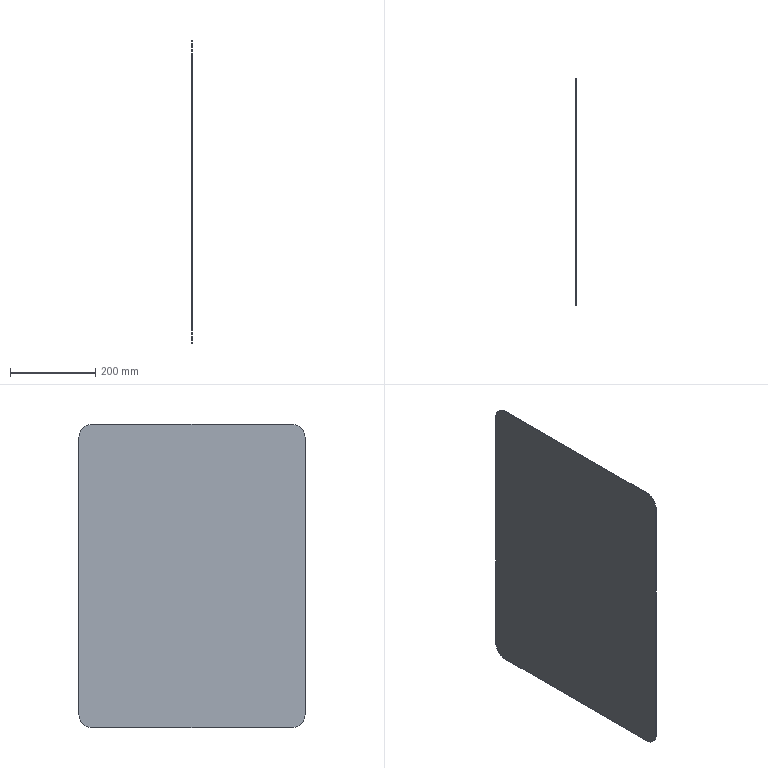Part | STEP file | 冲床-300配套压波_id1018_x_t | 1 solid | 10 faces | box 1.2 x 530 x 710 mm | volume 450633 mm3 | plane 6 | cylinder 4 | commonest cylinder face diameters 60 x4
STEP:
#1=CARTESIAN_POINT('',(1160.,-265.,-725.));
#2=VERTEX_POINT('',#1);
#3=CARTESIAN_POINT('',(1160.,-265.,-75.));
#4=VERTEX_POINT('',#3);
#5=CARTESIAN_POINT('',(1160.,-265.,-755.));
#6=DIRECTION('',(0.,0.,1.));
#7=VECTOR('',#6,1.);
#8=LINE('',#5,#7);
#9=EDGE_CURVE('',#2,#4,#8,.T.);
#10=ORIENTED_EDGE('',*,*,#9,.T.);
#11=CARTESIAN_POINT('',(1158.8,-265.,-75.));
#12=VERTEX_POINT('',#11);
#13=CARTESIAN_POINT('',(1160.,-265.,-75.));
#14=DIRECTION('',(-1.,0.,0.));
#15=VECTOR('',#14,1.);
#16=LINE('',#13,#15);
#17=EDGE_CURVE('',#4,#12,#16,.T.);
#18=ORIENTED_EDGE('',*,*,#17,.T.);
#19=CARTESIAN_POINT('',(1158.8,-265.,-725.));
#20=VERTEX_POINT('',#19);
#21=CARTESIAN_POINT('',(1158.8,-265.,-755.));
#22=DIRECTION('',(0.,0.,1.));
#23=VECTOR('',#22,1.);
#24=LINE('',#21,#23);
#25=EDGE_CURVE('',#20,#12,#24,.T.);
#26=ORIENTED_EDGE('',*,*,#25,.F.);
#27=CARTESIAN_POINT('',(1160.,-265.,-725.));
#28=DIRECTION('',(1.,0.,0.));
#29=VECTOR('',#28,1.);
#30=LINE('',#27,#29);
#31=EDGE_CURVE('',#20,#2,#30,.T.);
#32=ORIENTED_EDGE('',*,*,#31,.T.);
#33=EDGE_LOOP('',(#10,#18,#26,#32));
#34=FACE_OUTER_BOUND('',#33,.T.);
#35=CARTESIAN_POINT('',(1160.,-265.,-755.));
#36=DIRECTION('',(0.,-1.,0.));
#37=DIRECTION('',(0.,0.,-1.));
#38=AXIS2_PLACEMENT_3D('',#35,#36,#37);
#39=PLANE('',#38);
#40=ADVANCED_FACE('',(#34),#39,.T.);
#41=CARTESIAN_POINT('',(1160.,-235.,-45.));
#42=VERTEX_POINT('',#41);
#43=CARTESIAN_POINT('',(1160.,235.,-45.));
#44=VERTEX_POINT('',#43);
#45=CARTESIAN_POINT('',(1160.,-255.,-45.));
#46=DIRECTION('',(0.,1.,0.));
#47=VECTOR('',#46,1.);
#48=LINE('',#45,#47);
#49=EDGE_CURVE('',#42,#44,#48,.T.);
#50=ORIENTED_EDGE('',*,*,#49,.T.);
#51=CARTESIAN_POINT('',(1158.8,235.,-45.));
#52=VERTEX_POINT('',#51);
#53=CARTESIAN_POINT('',(1160.,235.,-45.));
#54=DIRECTION('',(-1.,0.,0.));
#55=VECTOR('',#54,1.);
#56=LINE('',#53,#55);
#57=EDGE_CURVE('',#44,#52,#56,.T.);
#58=ORIENTED_EDGE('',*,*,#57,.T.);
#59=CARTESIAN_POINT('',(1158.8,-235.,-45.));
#60=VERTEX_POINT('',#59);
#61=CARTESIAN_POINT('',(1158.8,-255.,-45.));
#62=DIRECTION('',(0.,1.,0.));
#63=VECTOR('',#62,1.);
#64=LINE('',#61,#63);
#65=EDGE_CURVE('',#60,#52,#64,.T.);
#66=ORIENTED_EDGE('',*,*,#65,.F.);
#67=CARTESIAN_POINT('',(1160.,-235.,-45.));
#68=DIRECTION('',(1.,0.,0.));
#69=VECTOR('',#68,1.);
#70=LINE('',#67,#69);
#71=EDGE_CURVE('',#60,#42,#70,.T.);
#72=ORIENTED_EDGE('',*,*,#71,.T.);
#73=EDGE_LOOP('',(#50,#58,#66,#72));
#74=FACE_OUTER_BOUND('',#73,.T.);
#75=CARTESIAN_POINT('',(1160.,-255.,-45.));
#76=DIRECTION('',(0.,0.,1.));
#77=DIRECTION('',(1.,0.,0.));
#78=AXIS2_PLACEMENT_3D('',#75,#76,#77);
#79=PLANE('',#78);
#80=ADVANCED_FACE('',(#74),#79,.T.);
#81=CARTESIAN_POINT('',(1160.,265.,-75.));
#82=VERTEX_POINT('',#81);
#83=CARTESIAN_POINT('',(1160.,265.,-725.));
#84=VERTEX_POINT('',#83);
#85=CARTESIAN_POINT('',(1160.,265.,-45.));
#86=DIRECTION('',(0.,0.,-1.));
#87=VECTOR('',#86,1.);
#88=LINE('',#85,#87);
#89=EDGE_CURVE('',#82,#84,#88,.T.);
#90=ORIENTED_EDGE('',*,*,#89,.T.);
#91=CARTESIAN_POINT('',(1158.8,265.,-725.));
#92=VERTEX_POINT('',#91);
#93=CARTESIAN_POINT('',(1160.,265.,-725.));
#94=DIRECTION('',(-1.,0.,0.));
#95=VECTOR('',#94,1.);
#96=LINE('',#93,#95);
#97=EDGE_CURVE('',#84,#92,#96,.T.);
#98=ORIENTED_EDGE('',*,*,#97,.T.);
#99=CARTESIAN_POINT('',(1158.8,265.,-75.));
#100=VERTEX_POINT('',#99);
#101=CARTESIAN_POINT('',(1158.8,265.,-45.));
#102=DIRECTION('',(0.,0.,-1.));
#103=VECTOR('',#102,1.);
#104=LINE('',#101,#103);
#105=EDGE_CURVE('',#100,#92,#104,.T.);
#106=ORIENTED_EDGE('',*,*,#105,.F.);
#107=CARTESIAN_POINT('',(1160.,265.,-75.));
#108=DIRECTION('',(1.,0.,0.));
#109=VECTOR('',#108,1.);
#110=LINE('',#107,#109);
#111=EDGE_CURVE('',#100,#82,#110,.T.);
#112=ORIENTED_EDGE('',*,*,#111,.T.);
#113=EDGE_LOOP('',(#90,#98,#106,#112));
#114=FACE_OUTER_BOUND('',#113,.T.);
#115=CARTESIAN_POINT('',(1160.,265.,-45.));
#116=DIRECTION('',(0.,1.,0.));
#117=DIRECTION('',(0.,0.,1.));
#118=AXIS2_PLACEMENT_3D('',#115,#116,#117);
#119=PLANE('',#118);
#120=ADVANCED_FACE('',(#114),#119,.T.);
#121=CARTESIAN_POINT('',(1158.8,235.,-755.));
#122=VERTEX_POINT('',#121);
#123=CARTESIAN_POINT('',(1158.8,-235.,-755.));
#124=VERTEX_POINT('',#123);
#125=CARTESIAN_POINT('',(1158.8,255.,-755.));
#126=DIRECTION('',(0.,-1.,0.));
#127=VECTOR('',#126,1.);
#128=LINE('',#125,#127);
#129=EDGE_CURVE('',#122,#124,#128,.T.);
#130=ORIENTED_EDGE('',*,*,#129,.F.);
#131=CARTESIAN_POINT('',(1160.,235.,-755.));
#132=VERTEX_POINT('',#131);
#133=CARTESIAN_POINT('',(1160.,235.,-755.));
#134=DIRECTION('',(1.,0.,0.));
#135=VECTOR('',#134,1.);
#136=LINE('',#133,#135);
#137=EDGE_CURVE('',#122,#132,#136,.T.);
#138=ORIENTED_EDGE('',*,*,#137,.T.);
#139=CARTESIAN_POINT('',(1160.,-235.,-755.));
#140=VERTEX_POINT('',#139);
#141=CARTESIAN_POINT('',(1160.,255.,-755.));
#142=DIRECTION('',(0.,-1.,0.));
#143=VECTOR('',#142,1.);
#144=LINE('',#141,#143);
#145=EDGE_CURVE('',#132,#140,#144,.T.);
#146=ORIENTED_EDGE('',*,*,#145,.T.);
#147=CARTESIAN_POINT('',(1160.,-235.,-755.));
#148=DIRECTION('',(-1.,0.,0.));
#149=VECTOR('',#148,1.);
#150=LINE('',#147,#149);
#151=EDGE_CURVE('',#140,#124,#150,.T.);
#152=ORIENTED_EDGE('',*,*,#151,.T.);
#153=EDGE_LOOP('',(#130,#138,#146,#152));
#154=FACE_OUTER_BOUND('',#153,.T.);
#155=CARTESIAN_POINT('',(1160.,255.,-755.));
#156=DIRECTION('',(0.,0.,-1.));
#157=DIRECTION('',(-1.,0.,0.));
#158=AXIS2_PLACEMENT_3D('',#155,#156,#157);
#159=PLANE('',#158);
#160=ADVANCED_FACE('',(#154),#159,.T.);
#161=ORIENTED_EDGE('',*,*,#145,.F.);
#162=CARTESIAN_POINT('',(1160.,235.,-725.));
#163=DIRECTION('',(1.,0.,0.));
#164=DIRECTION('',(0.,0.,1.));
#165=AXIS2_PLACEMENT_3D('',#162,#163,#164);
#166=CIRCLE('',#165,30.);
#167=EDGE_CURVE('',#132,#84,#166,.T.);
#168=ORIENTED_EDGE('',*,*,#167,.T.);
#169=ORIENTED_EDGE('',*,*,#89,.F.);
#170=CARTESIAN_POINT('',(1160.,235.,-75.));
#171=DIRECTION('',(1.,0.,0.));
#172=DIRECTION('',(0.,0.,1.));
#173=AXIS2_PLACEMENT_3D('',#170,#171,#172);
#174=CIRCLE('',#173,30.);
#175=EDGE_CURVE('',#82,#44,#174,.T.);
#176=ORIENTED_EDGE('',*,*,#175,.T.);
#177=ORIENTED_EDGE('',*,*,#49,.F.);
#178=CARTESIAN_POINT('',(1160.,-235.,-75.));
#179=DIRECTION('',(1.,0.,0.));
#180=DIRECTION('',(0.,0.,1.));
#181=AXIS2_PLACEMENT_3D('',#178,#179,#180);
#182=CIRCLE('',#181,30.);
#183=EDGE_CURVE('',#42,#4,#182,.T.);
#184=ORIENTED_EDGE('',*,*,#183,.T.);
#185=ORIENTED_EDGE('',*,*,#9,.F.);
#186=CARTESIAN_POINT('',(1160.,-235.,-725.));
#187=DIRECTION('',(1.,0.,0.));
#188=DIRECTION('',(0.,0.,1.));
#189=AXIS2_PLACEMENT_3D('',#186,#187,#188);
#190=CIRCLE('',#189,30.);
#191=EDGE_CURVE('',#2,#140,#190,.T.);
#192=ORIENTED_EDGE('',*,*,#191,.T.);
#193=EDGE_LOOP('',(#161,#168,#169,#176,#177,#184,#185,#192));
#194=FACE_OUTER_BOUND('',#193,.T.);
#195=CARTESIAN_POINT('',(1160.,0.,10.));
#196=DIRECTION('',(-1.,0.,0.));
#197=DIRECTION('',(0.,0.,1.));
#198=AXIS2_PLACEMENT_3D('',#195,#196,#197);
#199=PLANE('',#198);
#200=ADVANCED_FACE('',(#194),#199,.F.);
#201=ORIENTED_EDGE('',*,*,#105,.T.);
#202=CARTESIAN_POINT('',(1158.8,235.,-725.));
#203=DIRECTION('',(-1.,0.,0.));
#204=DIRECTION('',(0.,0.,1.));
#205=AXIS2_PLACEMENT_3D('',#202,#203,#204);
#206=CIRCLE('',#205,30.);
#207=EDGE_CURVE('',#92,#122,#206,.T.);
#208=ORIENTED_EDGE('',*,*,#207,.T.);
#209=ORIENTED_EDGE('',*,*,#129,.T.);
#210=CARTESIAN_POINT('',(1158.8,-235.,-725.));
#211=DIRECTION('',(-1.,0.,0.));
#212=DIRECTION('',(0.,0.,1.));
#213=AXIS2_PLACEMENT_3D('',#210,#211,#212);
#214=CIRCLE('',#213,30.);
#215=EDGE_CURVE('',#124,#20,#214,.T.);
#216=ORIENTED_EDGE('',*,*,#215,.T.);
#217=ORIENTED_EDGE('',*,*,#25,.T.);
#218=CARTESIAN_POINT('',(1158.8,-235.,-75.));
#219=DIRECTION('',(-1.,0.,0.));
#220=DIRECTION('',(0.,0.,1.));
#221=AXIS2_PLACEMENT_3D('',#218,#219,#220);
#222=CIRCLE('',#221,30.);
#223=EDGE_CURVE('',#12,#60,#222,.T.);
#224=ORIENTED_EDGE('',*,*,#223,.T.);
#225=ORIENTED_EDGE('',*,*,#65,.T.);
#226=CARTESIAN_POINT('',(1158.8,235.,-75.));
#227=DIRECTION('',(-1.,0.,0.));
#228=DIRECTION('',(0.,0.,1.));
#229=AXIS2_PLACEMENT_3D('',#226,#227,#228);
#230=CIRCLE('',#229,30.);
#231=EDGE_CURVE('',#52,#100,#230,.T.);
#232=ORIENTED_EDGE('',*,*,#231,.T.);
#233=EDGE_LOOP('',(#201,#208,#209,#216,#217,#224,#225,#232));
#234=FACE_OUTER_BOUND('',#233,.T.);
#235=CARTESIAN_POINT('',(1158.8,0.,10.));
#236=DIRECTION('',(-1.,0.,0.));
#237=DIRECTION('',(0.,0.,1.));
#238=AXIS2_PLACEMENT_3D('',#235,#236,#237);
#239=PLANE('',#238);
#240=ADVANCED_FACE('',(#234),#239,.T.);
#241=ORIENTED_EDGE('',*,*,#167,.F.);
#242=ORIENTED_EDGE('',*,*,#137,.F.);
#243=ORIENTED_EDGE('',*,*,#207,.F.);
#244=ORIENTED_EDGE('',*,*,#97,.F.);
#245=EDGE_LOOP('',(#241,#242,#243,#244));
#246=FACE_OUTER_BOUND('',#245,.T.);
#247=CARTESIAN_POINT('',(1160.,235.,-725.));
#248=DIRECTION('',(-1.,0.,0.));
#249=DIRECTION('',(0.,0.,1.));
#250=AXIS2_PLACEMENT_3D('',#247,#248,#249);
#251=CYLINDRICAL_SURFACE('',#250,30.);
#252=ADVANCED_FACE('',(#246),#251,.T.);
#253=ORIENTED_EDGE('',*,*,#175,.F.);
#254=ORIENTED_EDGE('',*,*,#111,.F.);
#255=ORIENTED_EDGE('',*,*,#231,.F.);
#256=ORIENTED_EDGE('',*,*,#57,.F.);
#257=EDGE_LOOP('',(#253,#254,#255,#256));
#258=FACE_OUTER_BOUND('',#257,.T.);
#259=CARTESIAN_POINT('',(1160.,235.,-75.));
#260=DIRECTION('',(-1.,0.,0.));
#261=DIRECTION('',(0.,0.,1.));
#262=AXIS2_PLACEMENT_3D('',#259,#260,#261);
#263=CYLINDRICAL_SURFACE('',#262,30.);
#264=ADVANCED_FACE('',(#258),#263,.T.);
#265=ORIENTED_EDGE('',*,*,#183,.F.);
#266=ORIENTED_EDGE('',*,*,#71,.F.);
#267=ORIENTED_EDGE('',*,*,#223,.F.);
#268=ORIENTED_EDGE('',*,*,#17,.F.);
#269=EDGE_LOOP('',(#265,#266,#267,#268));
#270=FACE_OUTER_BOUND('',#269,.T.);
#271=CARTESIAN_POINT('',(1160.,-235.,-75.));
#272=DIRECTION('',(-1.,0.,0.));
#273=DIRECTION('',(0.,0.,1.));
#274=AXIS2_PLACEMENT_3D('',#271,#272,#273);
#275=CYLINDRICAL_SURFACE('',#274,30.);
#276=ADVANCED_FACE('',(#270),#275,.T.);
#277=ORIENTED_EDGE('',*,*,#191,.F.);
#278=ORIENTED_EDGE('',*,*,#31,.F.);
#279=ORIENTED_EDGE('',*,*,#215,.F.);
#280=ORIENTED_EDGE('',*,*,#151,.F.);
#281=EDGE_LOOP('',(#277,#278,#279,#280));
#282=FACE_OUTER_BOUND('',#281,.T.);
#283=CARTESIAN_POINT('',(1160.,-235.,-725.));
#284=DIRECTION('',(-1.,0.,0.));
#285=DIRECTION('',(0.,0.,1.));
#286=AXIS2_PLACEMENT_3D('',#283,#284,#285);
#287=CYLINDRICAL_SURFACE('',#286,30.);
#288=ADVANCED_FACE('',(#282),#287,.T.);
#289=CLOSED_SHELL('',(#40,#80,#120,#160,#200,#240,#252,#264,#276,#288));
#290=MANIFOLD_SOLID_BREP('',#289);
#291=(LENGTH_UNIT()NAMED_UNIT(*)SI_UNIT(.MILLI.,.METRE.));
#292=UNCERTAINTY_MEASURE_WITH_UNIT(LENGTH_MEASURE(0.00002),#291,'','');
#293=(NAMED_UNIT(*)PLANE_ANGLE_UNIT()SI_UNIT($,.RADIAN.));
#294=PLANE_ANGLE_MEASURE_WITH_UNIT(PLANE_ANGLE_MEASURE(0.01745),#293);
#295=DIMENSIONAL_EXPONENTS(0.,0.,0.,0.,0.,0.,0.);
#296=(CONVERSION_BASED_UNIT('DEGREE',#294)NAMED_UNIT(#295)PLANE_ANGLE_UNIT());
#297=(NAMED_UNIT(*)SI_UNIT($,.STERADIAN.)SOLID_ANGLE_UNIT());
#298=(GEOMETRIC_REPRESENTATION_CONTEXT(3)GLOBAL_UNCERTAINTY_ASSIGNED_CONTEXT((#292))GLOBAL_UNIT_ASSIGNED_CONTEXT((#291,#296,#297))REPRESENTATION_CONTEXT('',''));
#299=ADVANCED_BREP_SHAPE_REPRESENTATION('',(#290),#298);